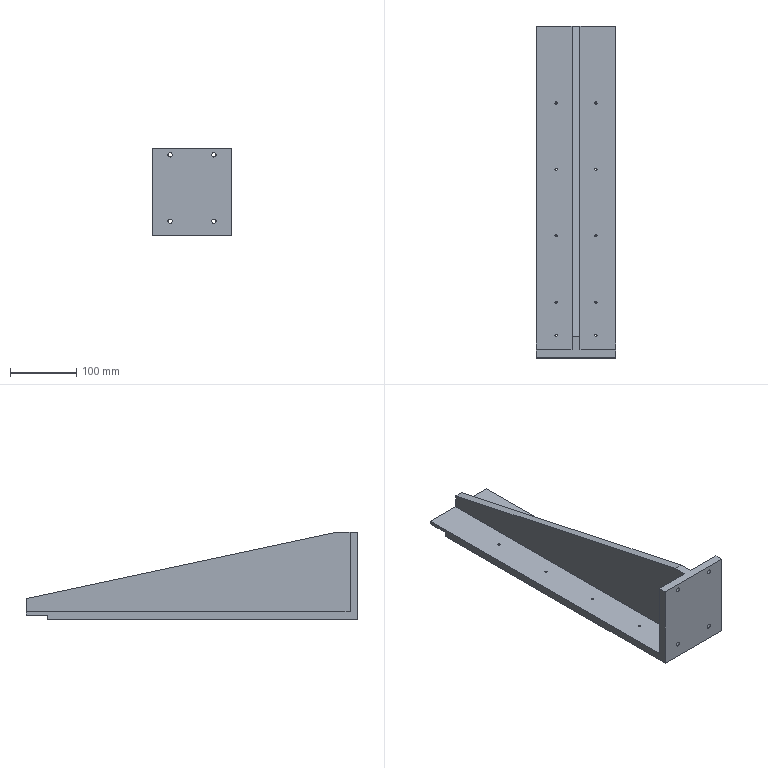Part | SolidWorks | features HoleWzd 3, ICE 2, Cut 1, Extrusion 1 | 1 solid | 43 faces | box 120 x 500 x 132 mm | volume 1285339 mm3 | cylinder 28 | plane 15 | commonest cylinder face diameters 3.3 x20 6.6 x8
STEP:
#1=CARTESIAN_POINT('',(28.35,34.,12.));
#2=VERTEX_POINT('',#1);
#3=CARTESIAN_POINT('',(31.65,34.,12.));
#4=VERTEX_POINT('',#3);
#5=CARTESIAN_POINT('',(30.,34.,12.));
#6=DIRECTION('',(0.,0.,1.));
#7=DIRECTION('',(1.,0.,0.));
#8=AXIS2_PLACEMENT_3D('',#5,#6,#7);
#9=CIRCLE('',#8,1.65);
#10=EDGE_CURVE('',#2,#4,#9,.T.);
#11=ORIENTED_EDGE('',*,*,#10,.T.);
#12=CARTESIAN_POINT('',(31.65,34.,0.));
#13=VERTEX_POINT('',#12);
#14=CARTESIAN_POINT('',(31.65,34.,0.));
#15=DIRECTION('',(0.,0.,-1.));
#16=VECTOR('',#15,1000.);
#17=LINE('',#14,#16);
#18=EDGE_CURVE('',#4,#13,#17,.T.);
#19=ORIENTED_EDGE('',*,*,#18,.T.);
#20=CARTESIAN_POINT('',(28.35,34.,0.));
#21=VERTEX_POINT('',#20);
#22=CARTESIAN_POINT('',(30.,34.,0.));
#23=DIRECTION('',(0.,0.,-1.));
#24=DIRECTION('',(-1.,0.,0.));
#25=AXIS2_PLACEMENT_3D('',#22,#23,#24);
#26=CIRCLE('',#25,1.65);
#27=EDGE_CURVE('',#13,#21,#26,.T.);
#28=ORIENTED_EDGE('',*,*,#27,.T.);
#29=CARTESIAN_POINT('',(28.35,34.,0.));
#30=DIRECTION('',(0.,0.,-1.));
#31=VECTOR('',#30,1000.);
#32=LINE('',#29,#31);
#33=EDGE_CURVE('',#2,#21,#32,.T.);
#34=ORIENTED_EDGE('',*,*,#33,.F.);
#35=EDGE_LOOP('',(#11,#19,#28,#34));
#36=FACE_OUTER_BOUND('',#35,.T.);
#37=CARTESIAN_POINT('',(30.,34.,0.));
#38=DIRECTION('',(0.,0.,-1.));
#39=DIRECTION('',(-1.,0.,0.));
#40=AXIS2_PLACEMENT_3D('',#37,#38,#39);
#41=CYLINDRICAL_SURFACE('',#40,1.65);
#42=ADVANCED_FACE('',(#36),#41,.F.);
#43=CARTESIAN_POINT('',(28.35,134.,12.));
#44=VERTEX_POINT('',#43);
#45=CARTESIAN_POINT('',(31.65,134.,12.));
#46=VERTEX_POINT('',#45);
#47=CARTESIAN_POINT('',(30.,134.,12.));
#48=DIRECTION('',(0.,0.,1.));
#49=DIRECTION('',(1.,0.,0.));
#50=AXIS2_PLACEMENT_3D('',#47,#48,#49);
#51=CIRCLE('',#50,1.65);
#52=EDGE_CURVE('',#44,#46,#51,.T.);
#53=ORIENTED_EDGE('',*,*,#52,.T.);
#54=CARTESIAN_POINT('',(31.65,134.,0.));
#55=VERTEX_POINT('',#54);
#56=CARTESIAN_POINT('',(31.65,134.,0.));
#57=DIRECTION('',(0.,0.,-1.));
#58=VECTOR('',#57,1000.);
#59=LINE('',#56,#58);
#60=EDGE_CURVE('',#46,#55,#59,.T.);
#61=ORIENTED_EDGE('',*,*,#60,.T.);
#62=CARTESIAN_POINT('',(28.35,134.,0.));
#63=VERTEX_POINT('',#62);
#64=CARTESIAN_POINT('',(30.,134.,0.));
#65=DIRECTION('',(0.,0.,-1.));
#66=DIRECTION('',(-1.,0.,0.));
#67=AXIS2_PLACEMENT_3D('',#64,#65,#66);
#68=CIRCLE('',#67,1.65);
#69=EDGE_CURVE('',#55,#63,#68,.T.);
#70=ORIENTED_EDGE('',*,*,#69,.T.);
#71=CARTESIAN_POINT('',(28.35,134.,0.));
#72=DIRECTION('',(0.,0.,-1.));
#73=VECTOR('',#72,1000.);
#74=LINE('',#71,#73);
#75=EDGE_CURVE('',#44,#63,#74,.T.);
#76=ORIENTED_EDGE('',*,*,#75,.F.);
#77=EDGE_LOOP('',(#53,#61,#70,#76));
#78=FACE_OUTER_BOUND('',#77,.T.);
#79=CARTESIAN_POINT('',(30.,134.,0.));
#80=DIRECTION('',(0.,0.,-1.));
#81=DIRECTION('',(-1.,0.,0.));
#82=AXIS2_PLACEMENT_3D('',#79,#80,#81);
#83=CYLINDRICAL_SURFACE('',#82,1.65);
#84=ADVANCED_FACE('',(#78),#83,.F.);
#85=CARTESIAN_POINT('',(28.35,-66.,12.));
#86=VERTEX_POINT('',#85);
#87=CARTESIAN_POINT('',(31.65,-66.,12.));
#88=VERTEX_POINT('',#87);
#89=CARTESIAN_POINT('',(30.,-66.,12.));
#90=DIRECTION('',(0.,0.,1.));
#91=DIRECTION('',(1.,0.,0.));
#92=AXIS2_PLACEMENT_3D('',#89,#90,#91);
#93=CIRCLE('',#92,1.65);
#94=EDGE_CURVE('',#86,#88,#93,.T.);
#95=ORIENTED_EDGE('',*,*,#94,.T.);
#96=CARTESIAN_POINT('',(31.65,-66.,0.));
#97=VERTEX_POINT('',#96);
#98=CARTESIAN_POINT('',(31.65,-66.,0.));
#99=DIRECTION('',(0.,0.,-1.));
#100=VECTOR('',#99,1000.);
#101=LINE('',#98,#100);
#102=EDGE_CURVE('',#88,#97,#101,.T.);
#103=ORIENTED_EDGE('',*,*,#102,.T.);
#104=CARTESIAN_POINT('',(28.35,-66.,0.));
#105=VERTEX_POINT('',#104);
#106=CARTESIAN_POINT('',(30.,-66.,0.));
#107=DIRECTION('',(0.,0.,-1.));
#108=DIRECTION('',(-1.,0.,0.));
#109=AXIS2_PLACEMENT_3D('',#106,#107,#108);
#110=CIRCLE('',#109,1.65);
#111=EDGE_CURVE('',#97,#105,#110,.T.);
#112=ORIENTED_EDGE('',*,*,#111,.T.);
#113=CARTESIAN_POINT('',(28.35,-66.,0.));
#114=DIRECTION('',(0.,0.,-1.));
#115=VECTOR('',#114,1000.);
#116=LINE('',#113,#115);
#117=EDGE_CURVE('',#86,#105,#116,.T.);
#118=ORIENTED_EDGE('',*,*,#117,.F.);
#119=EDGE_LOOP('',(#95,#103,#112,#118));
#120=FACE_OUTER_BOUND('',#119,.T.);
#121=CARTESIAN_POINT('',(30.,-66.,0.));
#122=DIRECTION('',(0.,0.,-1.));
#123=DIRECTION('',(-1.,0.,0.));
#124=AXIS2_PLACEMENT_3D('',#121,#122,#123);
#125=CYLINDRICAL_SURFACE('',#124,1.65);
#126=ADVANCED_FACE('',(#120),#125,.F.);
#127=CARTESIAN_POINT('',(28.35,-166.,12.));
#128=VERTEX_POINT('',#127);
#129=CARTESIAN_POINT('',(31.65,-166.,12.));
#130=VERTEX_POINT('',#129);
#131=CARTESIAN_POINT('',(30.,-166.,12.));
#132=DIRECTION('',(0.,0.,1.));
#133=DIRECTION('',(1.,0.,0.));
#134=AXIS2_PLACEMENT_3D('',#131,#132,#133);
#135=CIRCLE('',#134,1.65);
#136=EDGE_CURVE('',#128,#130,#135,.T.);
#137=ORIENTED_EDGE('',*,*,#136,.T.);
#138=CARTESIAN_POINT('',(31.65,-166.,0.));
#139=VERTEX_POINT('',#138);
#140=CARTESIAN_POINT('',(31.65,-166.,0.));
#141=DIRECTION('',(0.,0.,-1.));
#142=VECTOR('',#141,1000.);
#143=LINE('',#140,#142);
#144=EDGE_CURVE('',#130,#139,#143,.T.);
#145=ORIENTED_EDGE('',*,*,#144,.T.);
#146=CARTESIAN_POINT('',(28.35,-166.,0.));
#147=VERTEX_POINT('',#146);
#148=CARTESIAN_POINT('',(30.,-166.,0.));
#149=DIRECTION('',(0.,0.,-1.));
#150=DIRECTION('',(-1.,0.,0.));
#151=AXIS2_PLACEMENT_3D('',#148,#149,#150);
#152=CIRCLE('',#151,1.65);
#153=EDGE_CURVE('',#139,#147,#152,.T.);
#154=ORIENTED_EDGE('',*,*,#153,.T.);
#155=CARTESIAN_POINT('',(28.35,-166.,0.));
#156=DIRECTION('',(0.,0.,-1.));
#157=VECTOR('',#156,1000.);
#158=LINE('',#155,#157);
#159=EDGE_CURVE('',#128,#147,#158,.T.);
#160=ORIENTED_EDGE('',*,*,#159,.F.);
#161=EDGE_LOOP('',(#137,#145,#154,#160));
#162=FACE_OUTER_BOUND('',#161,.T.);
#163=CARTESIAN_POINT('',(30.,-166.,0.));
#164=DIRECTION('',(0.,0.,-1.));
#165=DIRECTION('',(-1.,0.,0.));
#166=AXIS2_PLACEMENT_3D('',#163,#164,#165);
#167=CYLINDRICAL_SURFACE('',#166,1.65);
#168=ADVANCED_FACE('',(#162),#167,.F.);
#169=CARTESIAN_POINT('',(28.35,-216.,12.));
#170=VERTEX_POINT('',#169);
#171=CARTESIAN_POINT('',(31.65,-216.,12.));
#172=VERTEX_POINT('',#171);
#173=CARTESIAN_POINT('',(30.,-216.,12.));
#174=DIRECTION('',(0.,0.,1.));
#175=DIRECTION('',(1.,0.,0.));
#176=AXIS2_PLACEMENT_3D('',#173,#174,#175);
#177=CIRCLE('',#176,1.65);
#178=EDGE_CURVE('',#170,#172,#177,.T.);
#179=ORIENTED_EDGE('',*,*,#178,.T.);
#180=CARTESIAN_POINT('',(31.65,-216.,0.));
#181=VERTEX_POINT('',#180);
#182=CARTESIAN_POINT('',(31.65,-216.,0.));
#183=DIRECTION('',(0.,0.,-1.));
#184=VECTOR('',#183,1000.);
#185=LINE('',#182,#184);
#186=EDGE_CURVE('',#172,#181,#185,.T.);
#187=ORIENTED_EDGE('',*,*,#186,.T.);
#188=CARTESIAN_POINT('',(28.35,-216.,0.));
#189=VERTEX_POINT('',#188);
#190=CARTESIAN_POINT('',(30.,-216.,0.));
#191=DIRECTION('',(0.,0.,-1.));
#192=DIRECTION('',(-1.,0.,0.));
#193=AXIS2_PLACEMENT_3D('',#190,#191,#192);
#194=CIRCLE('',#193,1.65);
#195=EDGE_CURVE('',#181,#189,#194,.T.);
#196=ORIENTED_EDGE('',*,*,#195,.T.);
#197=CARTESIAN_POINT('',(28.35,-216.,0.));
#198=DIRECTION('',(0.,0.,-1.));
#199=VECTOR('',#198,1000.);
#200=LINE('',#197,#199);
#201=EDGE_CURVE('',#170,#189,#200,.T.);
#202=ORIENTED_EDGE('',*,*,#201,.F.);
#203=EDGE_LOOP('',(#179,#187,#196,#202));
#204=FACE_OUTER_BOUND('',#203,.T.);
#205=CARTESIAN_POINT('',(30.,-216.,0.));
#206=DIRECTION('',(0.,0.,-1.));
#207=DIRECTION('',(-1.,0.,0.));
#208=AXIS2_PLACEMENT_3D('',#205,#206,#207);
#209=CYLINDRICAL_SURFACE('',#208,1.65);
#210=ADVANCED_FACE('',(#204),#209,.F.);
#211=CARTESIAN_POINT('',(-31.65,-216.,12.));
#212=VERTEX_POINT('',#211);
#213=CARTESIAN_POINT('',(-28.35,-216.,12.));
#214=VERTEX_POINT('',#213);
#215=CARTESIAN_POINT('',(-30.,-216.,12.));
#216=DIRECTION('',(0.,0.,1.));
#217=DIRECTION('',(1.,0.,0.));
#218=AXIS2_PLACEMENT_3D('',#215,#216,#217);
#219=CIRCLE('',#218,1.65);
#220=EDGE_CURVE('',#212,#214,#219,.T.);
#221=ORIENTED_EDGE('',*,*,#220,.T.);
#222=CARTESIAN_POINT('',(-28.35,-216.,0.));
#223=VERTEX_POINT('',#222);
#224=CARTESIAN_POINT('',(-28.35,-216.,0.));
#225=DIRECTION('',(0.,0.,-1.));
#226=VECTOR('',#225,1000.);
#227=LINE('',#224,#226);
#228=EDGE_CURVE('',#214,#223,#227,.T.);
#229=ORIENTED_EDGE('',*,*,#228,.T.);
#230=CARTESIAN_POINT('',(-31.65,-216.,0.));
#231=VERTEX_POINT('',#230);
#232=CARTESIAN_POINT('',(-30.,-216.,0.));
#233=DIRECTION('',(0.,0.,-1.));
#234=DIRECTION('',(-1.,0.,0.));
#235=AXIS2_PLACEMENT_3D('',#232,#233,#234);
#236=CIRCLE('',#235,1.65);
#237=EDGE_CURVE('',#223,#231,#236,.T.);
#238=ORIENTED_EDGE('',*,*,#237,.T.);
#239=CARTESIAN_POINT('',(-31.65,-216.,0.));
#240=DIRECTION('',(0.,0.,-1.));
#241=VECTOR('',#240,1000.);
#242=LINE('',#239,#241);
#243=EDGE_CURVE('',#212,#231,#242,.T.);
#244=ORIENTED_EDGE('',*,*,#243,.F.);
#245=EDGE_LOOP('',(#221,#229,#238,#244));
#246=FACE_OUTER_BOUND('',#245,.T.);
#247=CARTESIAN_POINT('',(-30.,-216.,0.));
#248=DIRECTION('',(0.,0.,-1.));
#249=DIRECTION('',(-1.,0.,0.));
#250=AXIS2_PLACEMENT_3D('',#247,#248,#249);
#251=CYLINDRICAL_SURFACE('',#250,1.65);
#252=ADVANCED_FACE('',(#246),#251,.F.);
#253=CARTESIAN_POINT('',(-31.65,-166.,12.));
#254=VERTEX_POINT('',#253);
#255=CARTESIAN_POINT('',(-28.35,-166.,12.));
#256=VERTEX_POINT('',#255);
#257=CARTESIAN_POINT('',(-30.,-166.,12.));
#258=DIRECTION('',(0.,0.,1.));
#259=DIRECTION('',(1.,0.,0.));
#260=AXIS2_PLACEMENT_3D('',#257,#258,#259);
#261=CIRCLE('',#260,1.65);
#262=EDGE_CURVE('',#254,#256,#261,.T.);
#263=ORIENTED_EDGE('',*,*,#262,.T.);
#264=CARTESIAN_POINT('',(-28.35,-166.,0.));
#265=VERTEX_POINT('',#264);
#266=CARTESIAN_POINT('',(-28.35,-166.,0.));
#267=DIRECTION('',(0.,0.,-1.));
#268=VECTOR('',#267,1000.);
#269=LINE('',#266,#268);
#270=EDGE_CURVE('',#256,#265,#269,.T.);
#271=ORIENTED_EDGE('',*,*,#270,.T.);
#272=CARTESIAN_POINT('',(-31.65,-166.,0.));
#273=VERTEX_POINT('',#272);
#274=CARTESIAN_POINT('',(-30.,-166.,0.));
#275=DIRECTION('',(0.,0.,-1.));
#276=DIRECTION('',(-1.,0.,0.));
#277=AXIS2_PLACEMENT_3D('',#274,#275,#276);
#278=CIRCLE('',#277,1.65);
#279=EDGE_CURVE('',#265,#273,#278,.T.);
#280=ORIENTED_EDGE('',*,*,#279,.T.);
#281=CARTESIAN_POINT('',(-31.65,-166.,0.));
#282=DIRECTION('',(0.,0.,-1.));
#283=VECTOR('',#282,1000.);
#284=LINE('',#281,#283);
#285=EDGE_CURVE('',#254,#273,#284,.T.);
#286=ORIENTED_EDGE('',*,*,#285,.F.);
#287=EDGE_LOOP('',(#263,#271,#280,#286));
#288=FACE_OUTER_BOUND('',#287,.T.);
#289=CARTESIAN_POINT('',(-30.,-166.,0.));
#290=DIRECTION('',(0.,0.,-1.));
#291=DIRECTION('',(-1.,0.,0.));
#292=AXIS2_PLACEMENT_3D('',#289,#290,#291);
#293=CYLINDRICAL_SURFACE('',#292,1.65);
#294=ADVANCED_FACE('',(#288),#293,.F.);
#295=CARTESIAN_POINT('',(-31.65,-66.,12.));
#296=VERTEX_POINT('',#295);
#297=CARTESIAN_POINT('',(-28.35,-66.,12.));
#298=VERTEX_POINT('',#297);
#299=CARTESIAN_POINT('',(-30.,-66.,12.));
#300=DIRECTION('',(0.,0.,1.));
#301=DIRECTION('',(1.,0.,0.));
#302=AXIS2_PLACEMENT_3D('',#299,#300,#301);
#303=CIRCLE('',#302,1.65);
#304=EDGE_CURVE('',#296,#298,#303,.T.);
#305=ORIENTED_EDGE('',*,*,#304,.T.);
#306=CARTESIAN_POINT('',(-28.35,-66.,0.));
#307=VERTEX_POINT('',#306);
#308=CARTESIAN_POINT('',(-28.35,-66.,0.));
#309=DIRECTION('',(0.,0.,-1.));
#310=VECTOR('',#309,1000.);
#311=LINE('',#308,#310);
#312=EDGE_CURVE('',#298,#307,#311,.T.);
#313=ORIENTED_EDGE('',*,*,#312,.T.);
#314=CARTESIAN_POINT('',(-31.65,-66.,0.));
#315=VERTEX_POINT('',#314);
#316=CARTESIAN_POINT('',(-30.,-66.,0.));
#317=DIRECTION('',(0.,0.,-1.));
#318=DIRECTION('',(-1.,0.,0.));
#319=AXIS2_PLACEMENT_3D('',#316,#317,#318);
#320=CIRCLE('',#319,1.65);
#321=EDGE_CURVE('',#307,#315,#320,.T.);
#322=ORIENTED_EDGE('',*,*,#321,.T.);
#323=CARTESIAN_POINT('',(-31.65,-66.,0.));
#324=DIRECTION('',(0.,0.,-1.));
#325=VECTOR('',#324,1000.);
#326=LINE('',#323,#325);
#327=EDGE_CURVE('',#296,#315,#326,.T.);
#328=ORIENTED_EDGE('',*,*,#327,.F.);
#329=EDGE_LOOP('',(#305,#313,#322,#328));
#330=FACE_OUTER_BOUND('',#329,.T.);
#331=CARTESIAN_POINT('',(-30.,-66.,0.));
#332=DIRECTION('',(0.,0.,-1.));
#333=DIRECTION('',(-1.,0.,0.));
#334=AXIS2_PLACEMENT_3D('',#331,#332,#333);
#335=CYLINDRICAL_SURFACE('',#334,1.65);
#336=ADVANCED_FACE('',(#330),#335,.F.);
#337=CARTESIAN_POINT('',(-31.65,34.,12.));
#338=VERTEX_POINT('',#337);
#339=CARTESIAN_POINT('',(-28.35,34.,12.));
#340=VERTEX_POINT('',#339);
#341=CARTESIAN_POINT('',(-30.,34.,12.));
#342=DIRECTION('',(0.,0.,1.));
#343=DIRECTION('',(1.,0.,0.));
#344=AXIS2_PLACEMENT_3D('',#341,#342,#343);
#345=CIRCLE('',#344,1.65);
#346=EDGE_CURVE('',#338,#340,#345,.T.);
#347=ORIENTED_EDGE('',*,*,#346,.T.);
#348=CARTESIAN_POINT('',(-28.35,34.,0.));
#349=VERTEX_POINT('',#348);
#350=CARTESIAN_POINT('',(-28.35,34.,0.));
#351=DIRECTION('',(0.,0.,-1.));
#352=VECTOR('',#351,1000.);
#353=LINE('',#350,#352);
#354=EDGE_CURVE('',#340,#349,#353,.T.);
#355=ORIENTED_EDGE('',*,*,#354,.T.);
#356=CARTESIAN_POINT('',(-31.65,34.,0.));
#357=VERTEX_POINT('',#356);
#358=CARTESIAN_POINT('',(-30.,34.,0.));
#359=DIRECTION('',(0.,0.,-1.));
#360=DIRECTION('',(-1.,0.,0.));
#361=AXIS2_PLACEMENT_3D('',#358,#359,#360);
#362=CIRCLE('',#361,1.65);
#363=EDGE_CURVE('',#349,#357,#362,.T.);
#364=ORIENTED_EDGE('',*,*,#363,.T.);
#365=CARTESIAN_POINT('',(-31.65,34.,0.));
#366=DIRECTION('',(0.,0.,-1.));
#367=VECTOR('',#366,1000.);
#368=LINE('',#365,#367);
#369=EDGE_CURVE('',#338,#357,#368,.T.);
#370=ORIENTED_EDGE('',*,*,#369,.F.);
#371=EDGE_LOOP('',(#347,#355,#364,#370));
#372=FACE_OUTER_BOUND('',#371,.T.);
#373=CARTESIAN_POINT('',(-30.,34.,0.));
#374=DIRECTION('',(0.,0.,-1.));
#375=DIRECTION('',(-1.,0.,0.));
#376=AXIS2_PLACEMENT_3D('',#373,#374,#375);
#377=CYLINDRICAL_SURFACE('',#376,1.65);
#378=ADVANCED_FACE('',(#372),#377,.F.);
#379=CARTESIAN_POINT('',(-31.65,134.,12.));
#380=VERTEX_POINT('',#379);
#381=CARTESIAN_POINT('',(-28.35,134.,12.));
#382=VERTEX_POINT('',#381);
#383=CARTESIAN_POINT('',(-30.,134.,12.));
#384=DIRECTION('',(0.,0.,1.));
#385=DIRECTION('',(1.,0.,0.));
#386=AXIS2_PLACEMENT_3D('',#383,#384,#385);
#387=CIRCLE('',#386,1.65);
#388=EDGE_CURVE('',#380,#382,#387,.T.);
#389=ORIENTED_EDGE('',*,*,#388,.T.);
#390=CARTESIAN_POINT('',(-28.35,134.,0.));
#391=VERTEX_POINT('',#390);
#392=CARTESIAN_POINT('',(-28.35,134.,0.));
#393=DIRECTION('',(0.,0.,-1.));
#394=VECTOR('',#393,1000.);
#395=LINE('',#392,#394);
#396=EDGE_CURVE('',#382,#391,#395,.T.);
#397=ORIENTED_EDGE('',*,*,#396,.T.);
#398=CARTESIAN_POINT('',(-31.65,134.,0.));
#399=VERTEX_POINT('',#398);
#400=CARTESIAN_POINT('',(-30.,134.,0.));
#401=DIRECTION('',(0.,0.,-1.));
#402=DIRECTION('',(-1.,0.,0.));
#403=AXIS2_PLACEMENT_3D('',#400,#401,#402);
#404=CIRCLE('',#403,1.65);
#405=EDGE_CURVE('',#391,#399,#404,.T.);
#406=ORIENTED_EDGE('',*,*,#405,.T.);
#407=CARTESIAN_POINT('',(-31.65,134.,0.));
#408=DIRECTION('',(0.,0.,-1.));
#409=VECTOR('',#408,1000.);
#410=LINE('',#407,#409);
#411=EDGE_CURVE('',#380,#399,#410,.T.);
#412=ORIENTED_EDGE('',*,*,#411,.F.);
#413=EDGE_LOOP('',(#389,#397,#406,#412));
#414=FACE_OUTER_BOUND('',#413,.T.);
#415=CARTESIAN_POINT('',(-30.,134.,0.));
#416=DIRECTION('',(0.,0.,-1.));
#417=DIRECTION('',(-1.,0.,0.));
#418=AXIS2_PLACEMENT_3D('',#415,#416,#417);
#419=CYLINDRICAL_SURFACE('',#418,1.65);
#420=ADVANCED_FACE('',(#414),#419,.F.);
#421=CARTESIAN_POINT('',(-33.,-250.,18.7));
#422=VERTEX_POINT('',#421);
#423=CARTESIAN_POINT('',(-33.,-250.,25.3));
#424=VERTEX_POINT('',#423);
#425=CARTESIAN_POINT('',(-33.,-250.,22.));
#426=DIRECTION('',(0.,1.,0.));
#427=DIRECTION('',(0.,0.,1.));
#428=AXIS2_PLACEMENT_3D('',#425,#426,#427);
#429=CIRCLE('',#428,3.3);
#430=EDGE_CURVE('',#422,#424,#429,.T.);
#431=ORIENTED_EDGE('',*,*,#430,.F.);
#432=CARTESIAN_POINT('',(-33.,-238.,18.7));
#433=VERTEX_POINT('',#432);
#434=CARTESIAN_POINT('',(-33.,-238.,18.7));
#435=DIRECTION('',(0.,1.,0.));
#436=VECTOR('',#435,1000.);
#437=LINE('',#434,#436);
#438=EDGE_CURVE('',#422,#433,#437,.T.);
#439=ORIENTED_EDGE('',*,*,#438,.T.);
#440=CARTESIAN_POINT('',(-33.,-238.,25.3));
#441=VERTEX_POINT('',#440);
#442=CARTESIAN_POINT('',(-33.,-238.,22.));
#443=DIRECTION('',(0.,1.,0.));
#444=DIRECTION('',(0.,0.,1.));
#445=AXIS2_PLACEMENT_3D('',#442,#443,#444);
#446=CIRCLE('',#445,3.3);
#447=EDGE_CURVE('',#433,#441,#446,.T.);
#448=ORIENTED_EDGE('',*,*,#447,.T.);
#449=CARTESIAN_POINT('',(-33.,-238.,25.3));
#450=DIRECTION('',(0.,1.,0.));
#451=VECTOR('',#450,1000.);
#452=LINE('',#449,#451);
#453=EDGE_CURVE('',#424,#441,#452,.T.);
#454=ORIENTED_EDGE('',*,*,#453,.F.);
#455=EDGE_LOOP('',(#431,#439,#448,#454));
#456=FACE_OUTER_BOUND('',#455,.T.);
#457=CARTESIAN_POINT('',(-33.,-238.,22.));
#458=DIRECTION('',(0.,1.,0.));
#459=DIRECTION('',(0.,0.,1.));
#460=AXIS2_PLACEMENT_3D('',#457,#458,#459);
#461=CYLINDRICAL_SURFACE('',#460,3.3);
#462=ADVANCED_FACE('',(#456),#461,.F.);
#463=CARTESIAN_POINT('',(-33.,-250.,118.7));
#464=VERTEX_POINT('',#463);
#465=CARTESIAN_POINT('',(-33.,-250.,125.3));
#466=VERTEX_POINT('',#465);
#467=CARTESIAN_POINT('',(-33.,-250.,122.));
#468=DIRECTION('',(0.,1.,0.));
#469=DIRECTION('',(0.,0.,1.));
#470=AXIS2_PLACEMENT_3D('',#467,#468,#469);
#471=CIRCLE('',#470,3.3);
#472=EDGE_CURVE('',#464,#466,#471,.T.);
#473=ORIENTED_EDGE('',*,*,#472,.F.);
#474=CARTESIAN_POINT('',(-33.,-238.,118.7));
#475=VERTEX_POINT('',#474);
#476=CARTESIAN_POINT('',(-33.,-238.,118.7));
#477=DIRECTION('',(0.,1.,0.));
#478=VECTOR('',#477,1000.);
#479=LINE('',#476,#478);
#480=EDGE_CURVE('',#464,#475,#479,.T.);
#481=ORIENTED_EDGE('',*,*,#480,.T.);
#482=CARTESIAN_POINT('',(-33.,-238.,125.3));
#483=VERTEX_POINT('',#482);
#484=CARTESIAN_POINT('',(-33.,-238.,122.));
#485=DIRECTION('',(0.,1.,0.));
#486=DIRECTION('',(0.,0.,1.));
#487=AXIS2_PLACEMENT_3D('',#484,#485,#486);
#488=CIRCLE('',#487,3.3);
#489=EDGE_CURVE('',#475,#483,#488,.T.);
#490=ORIENTED_EDGE('',*,*,#489,.T.);
#491=CARTESIAN_POINT('',(-33.,-238.,125.3));
#492=DIRECTION('',(0.,1.,0.));
#493=VECTOR('',#492,1000.);
#494=LINE('',#491,#493);
#495=EDGE_CURVE('',#466,#483,#494,.T.);
#496=ORIENTED_EDGE('',*,*,#495,.F.);
#497=EDGE_LOOP('',(#473,#481,#490,#496));
#498=FACE_OUTER_BOUND('',#497,.T.);
#499=CARTESIAN_POINT('',(-33.,-238.,122.));
#500=DIRECTION('',(0.,1.,0.));
#501=DIRECTION('',(0.,0.,1.));
#502=AXIS2_PLACEMENT_3D('',#499,#500,#501);
#503=CYLINDRICAL_SURFACE('',#502,3.3);
#504=ADVANCED_FACE('',(#498),#503,.F.);
#505=CARTESIAN_POINT('',(33.,-250.,18.7));
#506=VERTEX_POINT('',#505);
#507=CARTESIAN_POINT('',(33.,-250.,25.3));
#508=VERTEX_POINT('',#507);
#509=CARTESIAN_POINT('',(33.,-250.,22.));
#510=DIRECTION('',(0.,1.,0.));
#511=DIRECTION('',(0.,0.,1.));
#512=AXIS2_PLACEMENT_3D('',#509,#510,#511);
#513=CIRCLE('',#512,3.3);
#514=EDGE_CURVE('',#506,#508,#513,.T.);
#515=ORIENTED_EDGE('',*,*,#514,.F.);
#516=CARTESIAN_POINT('',(33.,-238.,18.7));
#517=VERTEX_POINT('',#516);
#518=CARTESIAN_POINT('',(33.,-238.,18.7));
#519=DIRECTION('',(0.,1.,0.));
#520=VECTOR('',#519,1000.);
#521=LINE('',#518,#520);
#522=EDGE_CURVE('',#506,#517,#521,.T.);
#523=ORIENTED_EDGE('',*,*,#522,.T.);
#524=CARTESIAN_POINT('',(33.,-238.,25.3));
#525=VERTEX_POINT('',#524);
#526=CARTESIAN_POINT('',(33.,-238.,22.));
#527=DIRECTION('',(0.,1.,0.));
#528=DIRECTION('',(0.,0.,1.));
#529=AXIS2_PLACEMENT_3D('',#526,#527,#528);
#530=CIRCLE('',#529,3.3);
#531=EDGE_CURVE('',#517,#525,#530,.T.);
#532=ORIENTED_EDGE('',*,*,#531,.T.);
#533=CARTESIAN_POINT('',(33.,-238.,25.3));
#534=DIRECTION('',(0.,1.,0.));
#535=VECTOR('',#534,1000.);
#536=LINE('',#533,#535);
#537=EDGE_CURVE('',#508,#525,#536,.T.);
#538=ORIENTED_EDGE('',*,*,#537,.F.);
#539=EDGE_LOOP('',(#515,#523,#532,#538));
#540=FACE_OUTER_BOUND('',#539,.T.);
#541=CARTESIAN_POINT('',(33.,-238.,22.));
#542=DIRECTION('',(0.,1.,0.));
#543=DIRECTION('',(0.,0.,1.));
#544=AXIS2_PLACEMENT_3D('',#541,#542,#543);
#545=CYLINDRICAL_SURFACE('',#544,3.3);
#546=ADVANCED_FACE('',(#540),#545,.F.);
#547=CARTESIAN_POINT('',(33.,-250.,118.7));
#548=VERTEX_POINT('',#547);
#549=CARTESIAN_POINT('',(33.,-250.,125.3));
#550=VERTEX_POINT('',#549);
#551=CARTESIAN_POINT('',(33.,-250.,122.));
#552=DIRECTION('',(0.,1.,0.));
#553=DIRECTION('',(0.,0.,1.));
#554=AXIS2_PLACEMENT_3D('',#551,#552,#553);
#555=CIRCLE('',#554,3.3);
#556=EDGE_CURVE('',#548,#550,#555,.T.);
#557=ORIENTED_EDGE('',*,*,#556,.F.);
#558=CARTESIAN_POINT('',(33.,-238.,118.7));
#559=VERTEX_POINT('',#558);
#560=CARTESIAN_POINT('',(33.,-238.,118.7));
#561=DIRECTION('',(0.,1.,0.));
#562=VECTOR('',#561,1000.);
#563=LINE('',#560,#562);
#564=EDGE_CURVE('',#548,#559,#563,.T.);
#565=ORIENTED_EDGE('',*,*,#564,.T.);
#566=CARTESIAN_POINT('',(33.,-238.,125.3));
#567=VERTEX_POINT('',#566);
#568=CARTESIAN_POINT('',(33.,-238.,122.));
#569=DIRECTION('',(0.,1.,0.));
#570=DIRECTION('',(0.,0.,1.));
#571=AXIS2_PLACEMENT_3D('',#568,#569,#570);
#572=CIRCLE('',#571,3.3);
#573=EDGE_CURVE('',#559,#567,#572,.T.);
#574=ORIENTED_EDGE('',*,*,#573,.T.);
#575=CARTESIAN_POINT('',(33.,-238.,125.3));
#576=DIRECTION('',(0.,1.,0.));
#577=VECTOR('',#576,1000.);
#578=LINE('',#575,#577);
#579=EDGE_CURVE('',#550,#567,#578,.T.);
#580=ORIENTED_EDGE('',*,*,#579,.F.);
#581=EDGE_LOOP('',(#557,#565,#574,#580));
#582=FACE_OUTER_BOUND('',#581,.T.);
#583=CARTESIAN_POINT('',(33.,-238.,122.));
#584=DIRECTION('',(0.,1.,0.));
#585=DIRECTION('',(0.,0.,1.));
#586=AXIS2_PLACEMENT_3D('',#583,#584,#585);
#587=CYLINDRICAL_SURFACE('',#586,3.3);
#588=ADVANCED_FACE('',(#582),#587,.F.);
#589=ORIENTED_EDGE('',*,*,#220,.F.);
#590=CARTESIAN_POINT('',(-30.,-216.,12.));
#591=DIRECTION('',(0.,0.,1.));
#592=DIRECTION('',(1.,0.,0.));
#593=AXIS2_PLACEMENT_3D('',#590,#591,#592);
#594=CIRCLE('',#593,1.65);
#595=EDGE_CURVE('',#214,#212,#594,.T.);
#596=ORIENTED_EDGE('',*,*,#595,.F.);
#597=EDGE_LOOP('',(#589,#596));
#598=FACE_BOUND('',#597,.T.);
#599=ORIENTED_EDGE('',*,*,#262,.F.);
#600=CARTESIAN_POINT('',(-30.,-166.,12.));
#601=DIRECTION('',(0.,0.,1.));
#602=DIRECTION('',(1.,0.,0.));
#603=AXIS2_PLACEMENT_3D('',#600,#601,#602);
#604=CIRCLE('',#603,1.65);
#605=EDGE_CURVE('',#256,#254,#604,.T.);
#606=ORIENTED_EDGE('',*,*,#605,.F.);
#607=EDGE_LOOP('',(#599,#606));
#608=FACE_BOUND('',#607,.T.);
#609=ORIENTED_EDGE('',*,*,#304,.F.);
#610=CARTESIAN_POINT('',(-30.,-66.,12.));
#611=DIRECTION('',(0.,0.,1.));
#612=DIRECTION('',(1.,0.,0.));
#613=AXIS2_PLACEMENT_3D('',#610,#611,#612);
#614=CIRCLE('',#613,1.65);
#615=EDGE_CURVE('',#298,#296,#614,.T.);
#616=ORIENTED_EDGE('',*,*,#615,.F.);
#617=EDGE_LOOP('',(#609,#616));
#618=FACE_BOUND('',#617,.T.);
#619=ORIENTED_EDGE('',*,*,#346,.F.);
#620=CARTESIAN_POINT('',(-30.,34.,12.));
#621=DIRECTION('',(0.,0.,1.));
#622=DIRECTION('',(1.,0.,0.));
#623=AXIS2_PLACEMENT_3D('',#620,#621,#622);
#624=CIRCLE('',#623,1.65);
#625=EDGE_CURVE('',#340,#338,#624,.T.);
#626=ORIENTED_EDGE('',*,*,#625,.F.);
#627=EDGE_LOOP('',(#619,#626));
#628=FACE_BOUND('',#627,.T.);
#629=ORIENTED_EDGE('',*,*,#388,.F.);
#630=CARTESIAN_POINT('',(-30.,134.,12.));
#631=DIRECTION('',(0.,0.,1.));
#632=DIRECTION('',(1.,0.,0.));
#633=AXIS2_PLACEMENT_3D('',#630,#631,#632);
#634=CIRCLE('',#633,1.65);
#635=EDGE_CURVE('',#382,#380,#634,.T.);
#636=ORIENTED_EDGE('',*,*,#635,.F.);
#637=EDGE_LOOP('',(#629,#636));
#638=FACE_BOUND('',#637,.T.);
#639=CARTESIAN_POINT('',(-6.,-238.,12.));
#640=VERTEX_POINT('',#639);
#641=CARTESIAN_POINT('',(-60.,-238.,12.));
#642=VERTEX_POINT('',#641);
#643=CARTESIAN_POINT('',(-60.,-238.,12.));
#644=DIRECTION('',(-1.,0.,0.));
#645=VECTOR('',#644,1000.);
#646=LINE('',#643,#645);
#647=EDGE_CURVE('',#640,#642,#646,.T.);
#648=ORIENTED_EDGE('',*,*,#647,.F.);
#649=CARTESIAN_POINT('',(-6.,250.,12.));
#650=VERTEX_POINT('',#649);
#651=CARTESIAN_POINT('',(-6.,-238.,12.));
#652=DIRECTION('',(0.,1.,0.));
#653=VECTOR('',#652,1000.);
#654=LINE('',#651,#653);
#655=EDGE_CURVE('',#640,#650,#654,.T.);
#656=ORIENTED_EDGE('',*,*,#655,.T.);
#657=CARTESIAN_POINT('',(-60.,250.,12.));
#658=VERTEX_POINT('',#657);
#659=CARTESIAN_POINT('',(-60.,250.,12.));
#660=DIRECTION('',(-1.,0.,0.));
#661=VECTOR('',#660,1000.);
#662=LINE('',#659,#661);
#663=EDGE_CURVE('',#650,#658,#662,.T.);
#664=ORIENTED_EDGE('',*,*,#663,.T.);
#665=CARTESIAN_POINT('',(-60.,250.,12.));
#666=DIRECTION('',(0.,-1.,0.));
#667=VECTOR('',#666,1000.);
#668=LINE('',#665,#667);
#669=EDGE_CURVE('',#658,#642,#668,.T.);
#670=ORIENTED_EDGE('',*,*,#669,.T.);
#671=EDGE_LOOP('',(#648,#656,#664,#670));
#672=FACE_OUTER_BOUND('',#671,.T.);
#673=CARTESIAN_POINT('',(0.,0.,12.));
#674=DIRECTION('',(0.,0.,1.));
#675=DIRECTION('',(1.,0.,0.));
#676=AXIS2_PLACEMENT_3D('',#673,#674,#675);
#677=PLANE('',#676);
#678=ADVANCED_FACE('',(#598,#608,#618,#628,#638,#672),#677,.T.);
#679=CARTESIAN_POINT('',(-33.,-238.,22.));
#680=DIRECTION('',(0.,1.,0.));
#681=DIRECTION('',(0.,0.,1.));
#682=AXIS2_PLACEMENT_3D('',#679,#680,#681);
#683=CIRCLE('',#682,3.3);
#684=EDGE_CURVE('',#441,#433,#683,.T.);
#685=ORIENTED_EDGE('',*,*,#684,.F.);
#686=ORIENTED_EDGE('',*,*,#447,.F.);
#687=EDGE_LOOP('',(#685,#686));
#688=FACE_BOUND('',#687,.T.);
#689=CARTESIAN_POINT('',(-33.,-238.,122.));
#690=DIRECTION('',(0.,1.,0.));
#691=DIRECTION('',(0.,0.,1.));
#692=AXIS2_PLACEMENT_3D('',#689,#690,#691);
#693=CIRCLE('',#692,3.3);
#694=EDGE_CURVE('',#483,#475,#693,.T.);
#695=ORIENTED_EDGE('',*,*,#694,.F.);
#696=ORIENTED_EDGE('',*,*,#489,.F.);
#697=EDGE_LOOP('',(#695,#696));
#698=FACE_BOUND('',#697,.T.);
#699=CARTESIAN_POINT('',(-6.,-238.,132.));
#700=VERTEX_POINT('',#699);
#701=CARTESIAN_POINT('',(-6.,-238.,132.));
#702=DIRECTION('',(0.,0.,-1.));
#703=VECTOR('',#702,1000.);
#704=LINE('',#701,#703);
#705=EDGE_CURVE('',#700,#640,#704,.T.);
#706=ORIENTED_EDGE('',*,*,#705,.T.);
#707=ORIENTED_EDGE('',*,*,#647,.T.);
#708=CARTESIAN_POINT('',(-60.,-238.,132.));
#709=VERTEX_POINT('',#708);
#710=CARTESIAN_POINT('',(-60.,-238.,132.));
#711=DIRECTION('',(0.,0.,-1.));
#712=VECTOR('',#711,1000.);
#713=LINE('',#710,#712);
#714=EDGE_CURVE('',#709,#642,#713,.T.);
#715=ORIENTED_EDGE('',*,*,#714,.F.);
#716=CARTESIAN_POINT('',(-60.,-238.,132.));
#717=DIRECTION('',(-1.,0.,0.));
#718=VECTOR('',#717,1000.);
#719=LINE('',#716,#718);
#720=EDGE_CURVE('',#700,#709,#719,.T.);
#721=ORIENTED_EDGE('',*,*,#720,.F.);
#722=EDGE_LOOP('',(#706,#707,#715,#721));
#723=FACE_OUTER_BOUND('',#722,.T.);
#724=CARTESIAN_POINT('',(-60.,-238.,132.));
#725=DIRECTION('',(0.,-1.,0.));
#726=DIRECTION('',(0.,0.,-1.));
#727=AXIS2_PLACEMENT_3D('',#724,#725,#726);
#728=PLANE('',#727);
#729=ADVANCED_FACE('',(#688,#698,#723),#728,.F.);
#730=CARTESIAN_POINT('',(60.,-250.,0.));
#731=VERTEX_POINT('',#730);
#732=CARTESIAN_POINT('',(60.,218.2,0.));
#733=VERTEX_POINT('',#732);
#734=CARTESIAN_POINT('',(60.,250.,0.));
#735=DIRECTION('',(0.,1.,0.));
#736=VECTOR('',#735,1000.);
#737=LINE('',#734,#736);
#738=EDGE_CURVE('',#731,#733,#737,.T.);
#739=ORIENTED_EDGE('',*,*,#738,.T.);
#740=CARTESIAN_POINT('',(60.,218.2,7.));
#741=VERTEX_POINT('',#740);
#742=CARTESIAN_POINT('',(60.,218.2,12.));
#743=DIRECTION('',(0.,0.,1.));
#744=VECTOR('',#743,1000.);
#745=LINE('',#742,#744);
#746=EDGE_CURVE('',#733,#741,#745,.T.);
#747=ORIENTED_EDGE('',*,*,#746,.T.);
#748=CARTESIAN_POINT('',(60.,250.,7.));
#749=VERTEX_POINT('',#748);
#750=CARTESIAN_POINT('',(60.,250.,7.));
#751=DIRECTION('',(0.,1.,0.));
#752=VECTOR('',#751,1000.);
#753=LINE('',#750,#752);
#754=EDGE_CURVE('',#741,#749,#753,.T.);
#755=ORIENTED_EDGE('',*,*,#754,.T.);
#756=CARTESIAN_POINT('',(60.,250.,12.));
#757=VERTEX_POINT('',#756);
#758=CARTESIAN_POINT('',(60.,250.,12.));
#759=DIRECTION('',(0.,0.,-1.));
#760=VECTOR('',#759,1000.);
#761=LINE('',#758,#760);
#762=EDGE_CURVE('',#757,#749,#761,.T.);
#763=ORIENTED_EDGE('',*,*,#762,.F.);
#764=CARTESIAN_POINT('',(60.,-238.,12.));
#765=VERTEX_POINT('',#764);
#766=CARTESIAN_POINT('',(60.,250.,12.));
#767=DIRECTION('',(0.,1.,0.));
#768=VECTOR('',#767,1000.);
#769=LINE('',#766,#768);
#770=EDGE_CURVE('',#765,#757,#769,.T.);
#771=ORIENTED_EDGE('',*,*,#770,.F.);
#772=CARTESIAN_POINT('',(60.,-238.,132.));
#773=VERTEX_POINT('',#772);
#774=CARTESIAN_POINT('',(60.,-238.,132.));
#775=DIRECTION('',(0.,0.,-1.));
#776=VECTOR('',#775,1000.);
#777=LINE('',#774,#776);
#778=EDGE_CURVE('',#773,#765,#777,.T.);
#779=ORIENTED_EDGE('',*,*,#778,.F.);
#780=CARTESIAN_POINT('',(60.,-250.,132.));
#781=VERTEX_POINT('',#780);
#782=CARTESIAN_POINT('',(60.,-250.,132.));
#783=DIRECTION('',(0.,1.,0.));
#784=VECTOR('',#783,1000.);
#785=LINE('',#782,#784);
#786=EDGE_CURVE('',#781,#773,#785,.T.);
#787=ORIENTED_EDGE('',*,*,#786,.F.);
#788=CARTESIAN_POINT('',(60.,-250.,12.));
#789=DIRECTION('',(0.,0.,-1.));
#790=VECTOR('',#789,1000.);
#791=LINE('',#788,#790);
#792=EDGE_CURVE('',#781,#731,#791,.T.);
#793=ORIENTED_EDGE('',*,*,#792,.T.);
#794=EDGE_LOOP('',(#739,#747,#755,#763,#771,#779,#787,#793));
#795=FACE_OUTER_BOUND('',#794,.T.);
#796=CARTESIAN_POINT('',(60.,250.,12.));
#797=DIRECTION('',(-1.,0.,0.));
#798=DIRECTION('',(0.,-1.,0.));
#799=AXIS2_PLACEMENT_3D('',#796,#797,#798);
#800=PLANE('',#799);
#801=ADVANCED_FACE('',(#795),#800,.F.);
#802=ORIENTED_EDGE('',*,*,#762,.T.);
#803=CARTESIAN_POINT('',(-60.,250.,7.));
#804=VERTEX_POINT('',#803);
#805=CARTESIAN_POINT('',(-60.,250.,7.));
#806=DIRECTION('',(1.,0.,0.));
#807=VECTOR('',#806,1000.);
#808=LINE('',#805,#807);
#809=EDGE_CURVE('',#804,#749,#808,.T.);
#810=ORIENTED_EDGE('',*,*,#809,.F.);
#811=CARTESIAN_POINT('',(-60.,250.,12.));
#812=DIRECTION('',(0.,0.,-1.));
#813=VECTOR('',#812,1000.);
#814=LINE('',#811,#813);
#815=EDGE_CURVE('',#658,#804,#814,.T.);
#816=ORIENTED_EDGE('',*,*,#815,.F.);
#817=ORIENTED_EDGE('',*,*,#663,.F.);
#818=CARTESIAN_POINT('',(-6.,250.,32.));
#819=VERTEX_POINT('',#818);
#820=CARTESIAN_POINT('',(-6.,250.,12.));
#821=DIRECTION('',(0.,0.,1.));
#822=VECTOR('',#821,1000.);
#823=LINE('',#820,#822);
#824=EDGE_CURVE('',#650,#819,#823,.T.);
#825=ORIENTED_EDGE('',*,*,#824,.T.);
#826=CARTESIAN_POINT('',(6.,250.,32.));
#827=VERTEX_POINT('',#826);
#828=CARTESIAN_POINT('',(6.,250.,32.));
#829=DIRECTION('',(-1.,0.,0.));
#830=VECTOR('',#829,1000.);
#831=LINE('',#828,#830);
#832=EDGE_CURVE('',#827,#819,#831,.T.);
#833=ORIENTED_EDGE('',*,*,#832,.F.);
#834=CARTESIAN_POINT('',(6.,250.,12.));
#835=VERTEX_POINT('',#834);
#836=CARTESIAN_POINT('',(6.,250.,12.));
#837=DIRECTION('',(0.,0.,1.));
#838=VECTOR('',#837,1000.);
#839=LINE('',#836,#838);
#840=EDGE_CURVE('',#835,#827,#839,.T.);
#841=ORIENTED_EDGE('',*,*,#840,.F.);
#842=CARTESIAN_POINT('',(-60.,250.,12.));
#843=DIRECTION('',(-1.,0.,0.));
#844=VECTOR('',#843,1000.);
#845=LINE('',#842,#844);
#846=EDGE_CURVE('',#757,#835,#845,.T.);
#847=ORIENTED_EDGE('',*,*,#846,.F.);
#848=EDGE_LOOP('',(#802,#810,#816,#817,#825,#833,#841,#847));
#849=FACE_OUTER_BOUND('',#848,.T.);
#850=CARTESIAN_POINT('',(-60.,250.,12.));
#851=DIRECTION('',(0.,-1.,0.));
#852=DIRECTION('',(0.,0.,-1.));
#853=AXIS2_PLACEMENT_3D('',#850,#851,#852);
#854=PLANE('',#853);
#855=ADVANCED_FACE('',(#849),#854,.F.);
#856=CARTESIAN_POINT('',(-60.,218.2,7.));
#857=VERTEX_POINT('',#856);
#858=CARTESIAN_POINT('',(-60.,250.,7.));
#859=DIRECTION('',(0.,-1.,0.));
#860=VECTOR('',#859,1000.);
#861=LINE('',#858,#860);
#862=EDGE_CURVE('',#804,#857,#861,.T.);
#863=ORIENTED_EDGE('',*,*,#862,.T.);
#864=CARTESIAN_POINT('',(-60.,218.2,0.));
#865=VERTEX_POINT('',#864);
#866=CARTESIAN_POINT('',(-60.,218.2,0.));
#867=DIRECTION('',(0.,0.,-1.));
#868=VECTOR('',#867,1000.);
#869=LINE('',#866,#868);
#870=EDGE_CURVE('',#857,#865,#869,.T.);
#871=ORIENTED_EDGE('',*,*,#870,.T.);
#872=CARTESIAN_POINT('',(-60.,-250.,0.));
#873=VERTEX_POINT('',#872);
#874=CARTESIAN_POINT('',(-60.,250.,0.));
#875=DIRECTION('',(0.,-1.,0.));
#876=VECTOR('',#875,1000.);
#877=LINE('',#874,#876);
#878=EDGE_CURVE('',#865,#873,#877,.T.);
#879=ORIENTED_EDGE('',*,*,#878,.T.);
#880=CARTESIAN_POINT('',(-60.,-250.,132.));
#881=VERTEX_POINT('',#880);
#882=CARTESIAN_POINT('',(-60.,-250.,12.));
#883=DIRECTION('',(0.,0.,-1.));
#884=VECTOR('',#883,1000.);
#885=LINE('',#882,#884);
#886=EDGE_CURVE('',#881,#873,#885,.T.);
#887=ORIENTED_EDGE('',*,*,#886,.F.);
#888=CARTESIAN_POINT('',(-60.,-250.,132.));
#889=DIRECTION('',(0.,-1.,0.));
#890=VECTOR('',#889,1000.);
#891=LINE('',#888,#890);
#892=EDGE_CURVE('',#709,#881,#891,.T.);
#893=ORIENTED_EDGE('',*,*,#892,.F.);
#894=ORIENTED_EDGE('',*,*,#714,.T.);
#895=ORIENTED_EDGE('',*,*,#669,.F.);
#896=ORIENTED_EDGE('',*,*,#815,.T.);
#897=EDGE_LOOP('',(#863,#871,#879,#887,#893,#894,#895,#896));
#898=FACE_OUTER_BOUND('',#897,.T.);
#899=CARTESIAN_POINT('',(-60.,250.,12.));
#900=DIRECTION('',(1.,0.,0.));
#901=DIRECTION('',(0.,1.,0.));
#902=AXIS2_PLACEMENT_3D('',#899,#900,#901);
#903=PLANE('',#902);
#904=ADVANCED_FACE('',(#898),#903,.F.);
#905=CARTESIAN_POINT('',(-33.,-250.,22.));
#906=DIRECTION('',(0.,1.,0.));
#907=DIRECTION('',(0.,0.,1.));
#908=AXIS2_PLACEMENT_3D('',#905,#906,#907);
#909=CIRCLE('',#908,3.3);
#910=EDGE_CURVE('',#424,#422,#909,.T.);
#911=ORIENTED_EDGE('',*,*,#910,.T.);
#912=ORIENTED_EDGE('',*,*,#430,.T.);
#913=EDGE_LOOP('',(#911,#912));
#914=FACE_BOUND('',#913,.T.);
#915=CARTESIAN_POINT('',(-33.,-250.,122.));
#916=DIRECTION('',(0.,1.,0.));
#917=DIRECTION('',(0.,0.,1.));
#918=AXIS2_PLACEMENT_3D('',#915,#916,#917);
#919=CIRCLE('',#918,3.3);
#920=EDGE_CURVE('',#466,#464,#919,.T.);
#921=ORIENTED_EDGE('',*,*,#920,.T.);
#922=ORIENTED_EDGE('',*,*,#472,.T.);
#923=EDGE_LOOP('',(#921,#922));
#924=FACE_BOUND('',#923,.T.);
#925=CARTESIAN_POINT('',(33.,-250.,22.));
#926=DIRECTION('',(0.,1.,0.));
#927=DIRECTION('',(0.,0.,1.));
#928=AXIS2_PLACEMENT_3D('',#925,#926,#927);
#929=CIRCLE('',#928,3.3);
#930=EDGE_CURVE('',#508,#506,#929,.T.);
#931=ORIENTED_EDGE('',*,*,#930,.T.);
#932=ORIENTED_EDGE('',*,*,#514,.T.);
#933=EDGE_LOOP('',(#931,#932));
#934=FACE_BOUND('',#933,.T.);
#935=CARTESIAN_POINT('',(33.,-250.,122.));
#936=DIRECTION('',(0.,1.,0.));
#937=DIRECTION('',(0.,0.,1.));
#938=AXIS2_PLACEMENT_3D('',#935,#936,#937);
#939=CIRCLE('',#938,3.3);
#940=EDGE_CURVE('',#550,#548,#939,.T.);
#941=ORIENTED_EDGE('',*,*,#940,.T.);
#942=ORIENTED_EDGE('',*,*,#556,.T.);
#943=EDGE_LOOP('',(#941,#942));
#944=FACE_BOUND('',#943,.T.);
#945=CARTESIAN_POINT('',(-60.,-250.,0.));
#946=DIRECTION('',(1.,0.,0.));
#947=VECTOR('',#946,1000.);
#948=LINE('',#945,#947);
#949=EDGE_CURVE('',#873,#731,#948,.T.);
#950=ORIENTED_EDGE('',*,*,#949,.T.);
#951=ORIENTED_EDGE('',*,*,#792,.F.);
#952=CARTESIAN_POINT('',(-60.,-250.,132.));
#953=DIRECTION('',(1.,0.,0.));
#954=VECTOR('',#953,1000.);
#955=LINE('',#952,#954);
#956=EDGE_CURVE('',#881,#781,#955,.T.);
#957=ORIENTED_EDGE('',*,*,#956,.F.);
#958=ORIENTED_EDGE('',*,*,#886,.T.);
#959=EDGE_LOOP('',(#950,#951,#957,#958));
#960=FACE_OUTER_BOUND('',#959,.T.);
#961=CARTESIAN_POINT('',(-60.,-250.,12.));
#962=DIRECTION('',(0.,1.,0.));
#963=DIRECTION('',(0.,0.,1.));
#964=AXIS2_PLACEMENT_3D('',#961,#962,#963);
#965=PLANE('',#964);
#966=ADVANCED_FACE('',(#914,#924,#934,#944,#960),#965,.F.);
#967=ORIENTED_EDGE('',*,*,#10,.F.);
#968=CARTESIAN_POINT('',(30.,34.,12.));
#969=DIRECTION('',(0.,0.,1.));
#970=DIRECTION('',(1.,0.,0.));
#971=AXIS2_PLACEMENT_3D('',#968,#969,#970);
#972=CIRCLE('',#971,1.65);
#973=EDGE_CURVE('',#4,#2,#972,.T.);
#974=ORIENTED_EDGE('',*,*,#973,.F.);
#975=EDGE_LOOP('',(#967,#974));
#976=FACE_BOUND('',#975,.T.);
#977=ORIENTED_EDGE('',*,*,#52,.F.);
#978=CARTESIAN_POINT('',(30.,134.,12.));
#979=DIRECTION('',(0.,0.,1.));
#980=DIRECTION('',(1.,0.,0.));
#981=AXIS2_PLACEMENT_3D('',#978,#979,#980);
#982=CIRCLE('',#981,1.65);
#983=EDGE_CURVE('',#46,#44,#982,.T.);
#984=ORIENTED_EDGE('',*,*,#983,.F.);
#985=EDGE_LOOP('',(#977,#984));
#986=FACE_BOUND('',#985,.T.);
#987=ORIENTED_EDGE('',*,*,#94,.F.);
#988=CARTESIAN_POINT('',(30.,-66.,12.));
#989=DIRECTION('',(0.,0.,1.));
#990=DIRECTION('',(1.,0.,0.));
#991=AXIS2_PLACEMENT_3D('',#988,#989,#990);
#992=CIRCLE('',#991,1.65);
#993=EDGE_CURVE('',#88,#86,#992,.T.);
#994=ORIENTED_EDGE('',*,*,#993,.F.);
#995=EDGE_LOOP('',(#987,#994));
#996=FACE_BOUND('',#995,.T.);
#997=ORIENTED_EDGE('',*,*,#136,.F.);
#998=CARTESIAN_POINT('',(30.,-166.,12.));
#999=DIRECTION('',(0.,0.,1.));
#1000=DIRECTION('',(1.,0.,0.));
#1001=AXIS2_PLACEMENT_3D('',#998,#999,#1000);
#1002=CIRCLE('',#1001,1.65);
#1003=EDGE_CURVE('',#130,#128,#1002,.T.);
#1004=ORIENTED_EDGE('',*,*,#1003,.F.);
#1005=EDGE_LOOP('',(#997,#1004));
#1006=FACE_BOUND('',#1005,.T.);
#1007=ORIENTED_EDGE('',*,*,#178,.F.);
#1008=CARTESIAN_POINT('',(30.,-216.,12.));
#1009=DIRECTION('',(0.,0.,1.));
#1010=DIRECTION('',(1.,0.,0.));
#1011=AXIS2_PLACEMENT_3D('',#1008,#1009,#1010);
#1012=CIRCLE('',#1011,1.65);
#1013=EDGE_CURVE('',#172,#170,#1012,.T.);
#1014=ORIENTED_EDGE('',*,*,#1013,.F.);
#1015=EDGE_LOOP('',(#1007,#1014));
#1016=FACE_BOUND('',#1015,.T.);
#1017=CARTESIAN_POINT('',(6.,-238.,12.));
#1018=VERTEX_POINT('',#1017);
#1019=CARTESIAN_POINT('',(6.,-238.,12.));
#1020=DIRECTION('',(0.,1.,0.));
#1021=VECTOR('',#1020,1000.);
#1022=LINE('',#1019,#1021);
#1023=EDGE_CURVE('',#1018,#835,#1022,.T.);
#1024=ORIENTED_EDGE('',*,*,#1023,.F.);
#1025=CARTESIAN_POINT('',(-60.,-238.,12.));
#1026=DIRECTION('',(-1.,0.,0.));
#1027=VECTOR('',#1026,1000.);
#1028=LINE('',#1025,#1027);
#1029=EDGE_CURVE('',#765,#1018,#1028,.T.);
#1030=ORIENTED_EDGE('',*,*,#1029,.F.);
#1031=ORIENTED_EDGE('',*,*,#770,.T.);
#1032=ORIENTED_EDGE('',*,*,#846,.T.);
#1033=EDGE_LOOP('',(#1024,#1030,#1031,#1032));
#1034=FACE_OUTER_BOUND('',#1033,.T.);
#1035=CARTESIAN_POINT('',(0.,0.,12.));
#1036=DIRECTION('',(0.,0.,1.));
#1037=DIRECTION('',(1.,0.,0.));
#1038=AXIS2_PLACEMENT_3D('',#1035,#1036,#1037);
#1039=PLANE('',#1038);
#1040=ADVANCED_FACE('',(#976,#986,#996,#1006,#1016,#1034),#1039,.T.);
#1041=CARTESIAN_POINT('',(30.,34.,0.));
#1042=DIRECTION('',(0.,0.,-1.));
#1043=DIRECTION('',(-1.,0.,0.));
#1044=AXIS2_PLACEMENT_3D('',#1041,#1042,#1043);
#1045=CIRCLE('',#1044,1.65);
#1046=EDGE_CURVE('',#21,#13,#1045,.T.);
#1047=ORIENTED_EDGE('',*,*,#1046,.F.);
#1048=ORIENTED_EDGE('',*,*,#27,.F.);
#1049=EDGE_LOOP('',(#1047,#1048));
#1050=FACE_BOUND('',#1049,.T.);
#1051=CARTESIAN_POINT('',(30.,134.,0.));
#1052=DIRECTION('',(0.,0.,-1.));
#1053=DIRECTION('',(-1.,0.,0.));
#1054=AXIS2_PLACEMENT_3D('',#1051,#1052,#1053);
#1055=CIRCLE('',#1054,1.65);
#1056=EDGE_CURVE('',#63,#55,#1055,.T.);
#1057=ORIENTED_EDGE('',*,*,#1056,.F.);
#1058=ORIENTED_EDGE('',*,*,#69,.F.);
#1059=EDGE_LOOP('',(#1057,#1058));
#1060=FACE_BOUND('',#1059,.T.);
#1061=CARTESIAN_POINT('',(30.,-66.,0.));
#1062=DIRECTION('',(0.,0.,-1.));
#1063=DIRECTION('',(-1.,0.,0.));
#1064=AXIS2_PLACEMENT_3D('',#1061,#1062,#1063);
#1065=CIRCLE('',#1064,1.65);
#1066=EDGE_CURVE('',#105,#97,#1065,.T.);
#1067=ORIENTED_EDGE('',*,*,#1066,.F.);
#1068=ORIENTED_EDGE('',*,*,#111,.F.);
#1069=EDGE_LOOP('',(#1067,#1068));
#1070=FACE_BOUND('',#1069,.T.);
#1071=CARTESIAN_POINT('',(30.,-166.,0.));
#1072=DIRECTION('',(0.,0.,-1.));
#1073=DIRECTION('',(-1.,0.,0.));
#1074=AXIS2_PLACEMENT_3D('',#1071,#1072,#1073);
#1075=CIRCLE('',#1074,1.65);
#1076=EDGE_CURVE('',#147,#139,#1075,.T.);
#1077=ORIENTED_EDGE('',*,*,#1076,.F.);
#1078=ORIENTED_EDGE('',*,*,#153,.F.);
#1079=EDGE_LOOP('',(#1077,#1078));
#1080=FACE_BOUND('',#1079,.T.);
#1081=CARTESIAN_POINT('',(30.,-216.,0.));
#1082=DIRECTION('',(0.,0.,-1.));
#1083=DIRECTION('',(-1.,0.,0.));
#1084=AXIS2_PLACEMENT_3D('',#1081,#1082,#1083);
#1085=CIRCLE('',#1084,1.65);
#1086=EDGE_CURVE('',#189,#181,#1085,.T.);
#1087=ORIENTED_EDGE('',*,*,#1086,.F.);
#1088=ORIENTED_EDGE('',*,*,#195,.F.);
#1089=EDGE_LOOP('',(#1087,#1088));
#1090=FACE_BOUND('',#1089,.T.);
#1091=CARTESIAN_POINT('',(-30.,-216.,0.));
#1092=DIRECTION('',(0.,0.,-1.));
#1093=DIRECTION('',(-1.,0.,0.));
#1094=AXIS2_PLACEMENT_3D('',#1091,#1092,#1093);
#1095=CIRCLE('',#1094,1.65);
#1096=EDGE_CURVE('',#231,#223,#1095,.T.);
#1097=ORIENTED_EDGE('',*,*,#1096,.F.);
#1098=ORIENTED_EDGE('',*,*,#237,.F.);
#1099=EDGE_LOOP('',(#1097,#1098));
#1100=FACE_BOUND('',#1099,.T.);
#1101=CARTESIAN_POINT('',(-30.,-166.,0.));
#1102=DIRECTION('',(0.,0.,-1.));
#1103=DIRECTION('',(-1.,0.,0.));
#1104=AXIS2_PLACEMENT_3D('',#1101,#1102,#1103);
#1105=CIRCLE('',#1104,1.65);
#1106=EDGE_CURVE('',#273,#265,#1105,.T.);
#1107=ORIENTED_EDGE('',*,*,#1106,.F.);
#1108=ORIENTED_EDGE('',*,*,#279,.F.);
#1109=EDGE_LOOP('',(#1107,#1108));
#1110=FACE_BOUND('',#1109,.T.);
#1111=CARTESIAN_POINT('',(-30.,-66.,0.));
#1112=DIRECTION('',(0.,0.,-1.));
#1113=DIRECTION('',(-1.,0.,0.));
#1114=AXIS2_PLACEMENT_3D('',#1111,#1112,#1113);
#1115=CIRCLE('',#1114,1.65);
#1116=EDGE_CURVE('',#315,#307,#1115,.T.);
#1117=ORIENTED_EDGE('',*,*,#1116,.F.);
#1118=ORIENTED_EDGE('',*,*,#321,.F.);
#1119=EDGE_LOOP('',(#1117,#1118));
#1120=FACE_BOUND('',#1119,.T.);
#1121=CARTESIAN_POINT('',(-30.,34.,0.));
#1122=DIRECTION('',(0.,0.,-1.));
#1123=DIRECTION('',(-1.,0.,0.));
#1124=AXIS2_PLACEMENT_3D('',#1121,#1122,#1123);
#1125=CIRCLE('',#1124,1.65);
#1126=EDGE_CURVE('',#357,#349,#1125,.T.);
#1127=ORIENTED_EDGE('',*,*,#1126,.F.);
#1128=ORIENTED_EDGE('',*,*,#363,.F.);
#1129=EDGE_LOOP('',(#1127,#1128));
#1130=FACE_BOUND('',#1129,.T.);
#1131=CARTESIAN_POINT('',(-30.,134.,0.));
#1132=DIRECTION('',(0.,0.,-1.));
#1133=DIRECTION('',(-1.,0.,0.));
#1134=AXIS2_PLACEMENT_3D('',#1131,#1132,#1133);
#1135=CIRCLE('',#1134,1.65);
#1136=EDGE_CURVE('',#399,#391,#1135,.T.);
#1137=ORIENTED_EDGE('',*,*,#1136,.F.);
#1138=ORIENTED_EDGE('',*,*,#405,.F.);
#1139=EDGE_LOOP('',(#1137,#1138));
#1140=FACE_BOUND('',#1139,.T.);
#1141=ORIENTED_EDGE('',*,*,#878,.F.);
#1142=CARTESIAN_POINT('',(-60.,218.2,0.));
#1143=DIRECTION('',(1.,0.,0.));
#1144=VECTOR('',#1143,1000.);
#1145=LINE('',#1142,#1144);
#1146=EDGE_CURVE('',#865,#733,#1145,.T.);
#1147=ORIENTED_EDGE('',*,*,#1146,.T.);
#1148=ORIENTED_EDGE('',*,*,#738,.F.);
#1149=ORIENTED_EDGE('',*,*,#949,.F.);
#1150=EDGE_LOOP('',(#1141,#1147,#1148,#1149));
#1151=FACE_OUTER_BOUND('',#1150,.T.);
#1152=CARTESIAN_POINT('',(0.,0.,0.));
#1153=DIRECTION('',(0.,0.,1.));
#1154=DIRECTION('',(1.,0.,0.));
#1155=AXIS2_PLACEMENT_3D('',#1152,#1153,#1154);
#1156=PLANE('',#1155);
#1157=ADVANCED_FACE('',(#1050,#1060,#1070,#1080,#1090,#1100,#1110,#1120,#1130,#1140,#1151),#1156,.F.);
#1158=CARTESIAN_POINT('',(33.,-238.,22.));
#1159=DIRECTION('',(0.,1.,0.));
#1160=DIRECTION('',(0.,0.,1.));
#1161=AXIS2_PLACEMENT_3D('',#1158,#1159,#1160);
#1162=CIRCLE('',#1161,3.3);
#1163=EDGE_CURVE('',#525,#517,#1162,.T.);
#1164=ORIENTED_EDGE('',*,*,#1163,.F.);
#1165=ORIENTED_EDGE('',*,*,#531,.F.);
#1166=EDGE_LOOP('',(#1164,#1165));
#1167=FACE_BOUND('',#1166,.T.);
#1168=CARTESIAN_POINT('',(33.,-238.,122.));
#1169=DIRECTION('',(0.,1.,0.));
#1170=DIRECTION('',(0.,0.,1.));
#1171=AXIS2_PLACEMENT_3D('',#1168,#1169,#1170);
#1172=CIRCLE('',#1171,3.3);
#1173=EDGE_CURVE('',#567,#559,#1172,.T.);
#1174=ORIENTED_EDGE('',*,*,#1173,.F.);
#1175=ORIENTED_EDGE('',*,*,#573,.F.);
#1176=EDGE_LOOP('',(#1174,#1175));
#1177=FACE_BOUND('',#1176,.T.);
#1178=ORIENTED_EDGE('',*,*,#1029,.T.);
#1179=CARTESIAN_POINT('',(6.,-238.,132.));
#1180=VERTEX_POINT('',#1179);
#1181=CARTESIAN_POINT('',(6.,-238.,132.));
#1182=DIRECTION('',(0.,0.,-1.));
#1183=VECTOR('',#1182,1000.);
#1184=LINE('',#1181,#1183);
#1185=EDGE_CURVE('',#1180,#1018,#1184,.T.);
#1186=ORIENTED_EDGE('',*,*,#1185,.F.);
#1187=CARTESIAN_POINT('',(-60.,-238.,132.));
#1188=DIRECTION('',(-1.,0.,0.));
#1189=VECTOR('',#1188,1000.);
#1190=LINE('',#1187,#1189);
#1191=EDGE_CURVE('',#773,#1180,#1190,.T.);
#1192=ORIENTED_EDGE('',*,*,#1191,.F.);
#1193=ORIENTED_EDGE('',*,*,#778,.T.);
#1194=EDGE_LOOP('',(#1178,#1186,#1192,#1193));
#1195=FACE_OUTER_BOUND('',#1194,.T.);
#1196=CARTESIAN_POINT('',(-60.,-238.,132.));
#1197=DIRECTION('',(0.,-1.,0.));
#1198=DIRECTION('',(0.,0.,-1.));
#1199=AXIS2_PLACEMENT_3D('',#1196,#1197,#1198);
#1200=PLANE('',#1199);
#1201=ADVANCED_FACE('',(#1167,#1177,#1195),#1200,.F.);
#1202=ORIENTED_EDGE('',*,*,#892,.T.);
#1203=ORIENTED_EDGE('',*,*,#956,.T.);
#1204=ORIENTED_EDGE('',*,*,#786,.T.);
#1205=ORIENTED_EDGE('',*,*,#1191,.T.);
#1206=CARTESIAN_POINT('',(6.,-218.,132.));
#1207=VERTEX_POINT('',#1206);
#1208=CARTESIAN_POINT('',(6.,-218.,132.));
#1209=DIRECTION('',(0.,-1.,0.));
#1210=VECTOR('',#1209,1000.);
#1211=LINE('',#1208,#1210);
#1212=EDGE_CURVE('',#1207,#1180,#1211,.T.);
#1213=ORIENTED_EDGE('',*,*,#1212,.F.);
#1214=CARTESIAN_POINT('',(-6.,-218.,132.));
#1215=VERTEX_POINT('',#1214);
#1216=CARTESIAN_POINT('',(6.,-218.,132.));
#1217=DIRECTION('',(-1.,0.,0.));
#1218=VECTOR('',#1217,1000.);
#1219=LINE('',#1216,#1218);
#1220=EDGE_CURVE('',#1207,#1215,#1219,.T.);
#1221=ORIENTED_EDGE('',*,*,#1220,.T.);
#1222=CARTESIAN_POINT('',(-6.,-218.,132.));
#1223=DIRECTION('',(0.,-1.,0.));
#1224=VECTOR('',#1223,1000.);
#1225=LINE('',#1222,#1224);
#1226=EDGE_CURVE('',#1215,#700,#1225,.T.);
#1227=ORIENTED_EDGE('',*,*,#1226,.T.);
#1228=ORIENTED_EDGE('',*,*,#720,.T.);
#1229=EDGE_LOOP('',(#1202,#1203,#1204,#1205,#1213,#1221,#1227,#1228));
#1230=FACE_OUTER_BOUND('',#1229,.T.);
#1231=CARTESIAN_POINT('',(0.,0.,132.));
#1232=DIRECTION('',(0.,0.,-1.));
#1233=DIRECTION('',(-1.,0.,0.));
#1234=AXIS2_PLACEMENT_3D('',#1231,#1232,#1233);
#1235=PLANE('',#1234);
#1236=ADVANCED_FACE('',(#1230),#1235,.F.);
#1237=CARTESIAN_POINT('',(-6.,250.,32.));
#1238=DIRECTION('',(0.,-0.9779,0.209));
#1239=VECTOR('',#1238,1000.);
#1240=LINE('',#1237,#1239);
#1241=EDGE_CURVE('',#819,#1215,#1240,.T.);
#1242=ORIENTED_EDGE('',*,*,#1241,.T.);
#1243=ORIENTED_EDGE('',*,*,#1220,.F.);
#1244=CARTESIAN_POINT('',(6.,250.,32.));
#1245=DIRECTION('',(0.,-0.9779,0.209));
#1246=VECTOR('',#1245,1000.);
#1247=LINE('',#1244,#1246);
#1248=EDGE_CURVE('',#827,#1207,#1247,.T.);
#1249=ORIENTED_EDGE('',*,*,#1248,.F.);
#1250=ORIENTED_EDGE('',*,*,#832,.T.);
#1251=EDGE_LOOP('',(#1242,#1243,#1249,#1250));
#1252=FACE_OUTER_BOUND('',#1251,.T.);
#1253=CARTESIAN_POINT('',(6.,250.,32.));
#1254=DIRECTION('',(0.,-0.209,-0.9779));
#1255=DIRECTION('',(0.,0.9779,-0.209));
#1256=AXIS2_PLACEMENT_3D('',#1253,#1254,#1255);
#1257=PLANE('',#1256);
#1258=ADVANCED_FACE('',(#1252),#1257,.F.);
#1259=ORIENTED_EDGE('',*,*,#1023,.T.);
#1260=ORIENTED_EDGE('',*,*,#840,.T.);
#1261=ORIENTED_EDGE('',*,*,#1248,.T.);
#1262=ORIENTED_EDGE('',*,*,#1212,.T.);
#1263=ORIENTED_EDGE('',*,*,#1185,.T.);
#1264=EDGE_LOOP('',(#1259,#1260,#1261,#1262,#1263));
#1265=FACE_OUTER_BOUND('',#1264,.T.);
#1266=CARTESIAN_POINT('',(6.,0.,0.));
#1267=DIRECTION('',(1.,0.,0.));
#1268=DIRECTION('',(0.,0.,-1.));
#1269=AXIS2_PLACEMENT_3D('',#1266,#1267,#1268);
#1270=PLANE('',#1269);
#1271=ADVANCED_FACE('',(#1265),#1270,.T.);
#1272=ORIENTED_EDGE('',*,*,#655,.F.);
#1273=ORIENTED_EDGE('',*,*,#705,.F.);
#1274=ORIENTED_EDGE('',*,*,#1226,.F.);
#1275=ORIENTED_EDGE('',*,*,#1241,.F.);
#1276=ORIENTED_EDGE('',*,*,#824,.F.);
#1277=EDGE_LOOP('',(#1272,#1273,#1274,#1275,#1276));
#1278=FACE_OUTER_BOUND('',#1277,.T.);
#1279=CARTESIAN_POINT('',(-6.,0.,0.));
#1280=DIRECTION('',(1.,0.,0.));
#1281=DIRECTION('',(0.,0.,-1.));
#1282=AXIS2_PLACEMENT_3D('',#1279,#1280,#1281);
#1283=PLANE('',#1282);
#1284=ADVANCED_FACE('',(#1278),#1283,.F.);
#1285=ORIENTED_EDGE('',*,*,#564,.F.);
#1286=ORIENTED_EDGE('',*,*,#940,.F.);
#1287=ORIENTED_EDGE('',*,*,#579,.T.);
#1288=ORIENTED_EDGE('',*,*,#1173,.T.);
#1289=EDGE_LOOP('',(#1285,#1286,#1287,#1288));
#1290=FACE_OUTER_BOUND('',#1289,.T.);
#1291=CARTESIAN_POINT('',(33.,-238.,122.));
#1292=DIRECTION('',(0.,1.,0.));
#1293=DIRECTION('',(0.,0.,1.));
#1294=AXIS2_PLACEMENT_3D('',#1291,#1292,#1293);
#1295=CYLINDRICAL_SURFACE('',#1294,3.3);
#1296=ADVANCED_FACE('',(#1290),#1295,.F.);
#1297=ORIENTED_EDGE('',*,*,#522,.F.);
#1298=ORIENTED_EDGE('',*,*,#930,.F.);
#1299=ORIENTED_EDGE('',*,*,#537,.T.);
#1300=ORIENTED_EDGE('',*,*,#1163,.T.);
#1301=EDGE_LOOP('',(#1297,#1298,#1299,#1300));
#1302=FACE_OUTER_BOUND('',#1301,.T.);
#1303=CARTESIAN_POINT('',(33.,-238.,22.));
#1304=DIRECTION('',(0.,1.,0.));
#1305=DIRECTION('',(0.,0.,1.));
#1306=AXIS2_PLACEMENT_3D('',#1303,#1304,#1305);
#1307=CYLINDRICAL_SURFACE('',#1306,3.3);
#1308=ADVANCED_FACE('',(#1302),#1307,.F.);
#1309=ORIENTED_EDGE('',*,*,#480,.F.);
#1310=ORIENTED_EDGE('',*,*,#920,.F.);
#1311=ORIENTED_EDGE('',*,*,#495,.T.);
#1312=ORIENTED_EDGE('',*,*,#694,.T.);
#1313=EDGE_LOOP('',(#1309,#1310,#1311,#1312));
#1314=FACE_OUTER_BOUND('',#1313,.T.);
#1315=CARTESIAN_POINT('',(-33.,-238.,122.));
#1316=DIRECTION('',(0.,1.,0.));
#1317=DIRECTION('',(0.,0.,1.));
#1318=AXIS2_PLACEMENT_3D('',#1315,#1316,#1317);
#1319=CYLINDRICAL_SURFACE('',#1318,3.3);
#1320=ADVANCED_FACE('',(#1314),#1319,.F.);
#1321=ORIENTED_EDGE('',*,*,#438,.F.);
#1322=ORIENTED_EDGE('',*,*,#910,.F.);
#1323=ORIENTED_EDGE('',*,*,#453,.T.);
#1324=ORIENTED_EDGE('',*,*,#684,.T.);
#1325=EDGE_LOOP('',(#1321,#1322,#1323,#1324));
#1326=FACE_OUTER_BOUND('',#1325,.T.);
#1327=CARTESIAN_POINT('',(-33.,-238.,22.));
#1328=DIRECTION('',(0.,1.,0.));
#1329=DIRECTION('',(0.,0.,1.));
#1330=AXIS2_PLACEMENT_3D('',#1327,#1328,#1329);
#1331=CYLINDRICAL_SURFACE('',#1330,3.3);
#1332=ADVANCED_FACE('',(#1326),#1331,.F.);
#1333=ORIENTED_EDGE('',*,*,#396,.F.);
#1334=ORIENTED_EDGE('',*,*,#635,.T.);
#1335=ORIENTED_EDGE('',*,*,#411,.T.);
#1336=ORIENTED_EDGE('',*,*,#1136,.T.);
#1337=EDGE_LOOP('',(#1333,#1334,#1335,#1336));
#1338=FACE_OUTER_BOUND('',#1337,.T.);
#1339=CARTESIAN_POINT('',(-30.,134.,0.));
#1340=DIRECTION('',(0.,0.,-1.));
#1341=DIRECTION('',(-1.,0.,0.));
#1342=AXIS2_PLACEMENT_3D('',#1339,#1340,#1341);
#1343=CYLINDRICAL_SURFACE('',#1342,1.65);
#1344=ADVANCED_FACE('',(#1338),#1343,.F.);
#1345=ORIENTED_EDGE('',*,*,#354,.F.);
#1346=ORIENTED_EDGE('',*,*,#625,.T.);
#1347=ORIENTED_EDGE('',*,*,#369,.T.);
#1348=ORIENTED_EDGE('',*,*,#1126,.T.);
#1349=EDGE_LOOP('',(#1345,#1346,#1347,#1348));
#1350=FACE_OUTER_BOUND('',#1349,.T.);
#1351=CARTESIAN_POINT('',(-30.,34.,0.));
#1352=DIRECTION('',(0.,0.,-1.));
#1353=DIRECTION('',(-1.,0.,0.));
#1354=AXIS2_PLACEMENT_3D('',#1351,#1352,#1353);
#1355=CYLINDRICAL_SURFACE('',#1354,1.65);
#1356=ADVANCED_FACE('',(#1350),#1355,.F.);
#1357=ORIENTED_EDGE('',*,*,#312,.F.);
#1358=ORIENTED_EDGE('',*,*,#615,.T.);
#1359=ORIENTED_EDGE('',*,*,#327,.T.);
#1360=ORIENTED_EDGE('',*,*,#1116,.T.);
#1361=EDGE_LOOP('',(#1357,#1358,#1359,#1360));
#1362=FACE_OUTER_BOUND('',#1361,.T.);
#1363=CARTESIAN_POINT('',(-30.,-66.,0.));
#1364=DIRECTION('',(0.,0.,-1.));
#1365=DIRECTION('',(-1.,0.,0.));
#1366=AXIS2_PLACEMENT_3D('',#1363,#1364,#1365);
#1367=CYLINDRICAL_SURFACE('',#1366,1.65);
#1368=ADVANCED_FACE('',(#1362),#1367,.F.);
#1369=ORIENTED_EDGE('',*,*,#270,.F.);
#1370=ORIENTED_EDGE('',*,*,#605,.T.);
#1371=ORIENTED_EDGE('',*,*,#285,.T.);
#1372=ORIENTED_EDGE('',*,*,#1106,.T.);
#1373=EDGE_LOOP('',(#1369,#1370,#1371,#1372));
#1374=FACE_OUTER_BOUND('',#1373,.T.);
#1375=CARTESIAN_POINT('',(-30.,-166.,0.));
#1376=DIRECTION('',(0.,0.,-1.));
#1377=DIRECTION('',(-1.,0.,0.));
#1378=AXIS2_PLACEMENT_3D('',#1375,#1376,#1377);
#1379=CYLINDRICAL_SURFACE('',#1378,1.65);
#1380=ADVANCED_FACE('',(#1374),#1379,.F.);
#1381=ORIENTED_EDGE('',*,*,#228,.F.);
#1382=ORIENTED_EDGE('',*,*,#595,.T.);
#1383=ORIENTED_EDGE('',*,*,#243,.T.);
#1384=ORIENTED_EDGE('',*,*,#1096,.T.);
#1385=EDGE_LOOP('',(#1381,#1382,#1383,#1384));
#1386=FACE_OUTER_BOUND('',#1385,.T.);
#1387=CARTESIAN_POINT('',(-30.,-216.,0.));
#1388=DIRECTION('',(0.,0.,-1.));
#1389=DIRECTION('',(-1.,0.,0.));
#1390=AXIS2_PLACEMENT_3D('',#1387,#1388,#1389);
#1391=CYLINDRICAL_SURFACE('',#1390,1.65);
#1392=ADVANCED_FACE('',(#1386),#1391,.F.);
#1393=ORIENTED_EDGE('',*,*,#186,.F.);
#1394=ORIENTED_EDGE('',*,*,#1013,.T.);
#1395=ORIENTED_EDGE('',*,*,#201,.T.);
#1396=ORIENTED_EDGE('',*,*,#1086,.T.);
#1397=EDGE_LOOP('',(#1393,#1394,#1395,#1396));
#1398=FACE_OUTER_BOUND('',#1397,.T.);
#1399=CARTESIAN_POINT('',(30.,-216.,0.));
#1400=DIRECTION('',(0.,0.,-1.));
#1401=DIRECTION('',(-1.,0.,0.));
#1402=AXIS2_PLACEMENT_3D('',#1399,#1400,#1401);
#1403=CYLINDRICAL_SURFACE('',#1402,1.65);
#1404=ADVANCED_FACE('',(#1398),#1403,.F.);
#1405=ORIENTED_EDGE('',*,*,#144,.F.);
#1406=ORIENTED_EDGE('',*,*,#1003,.T.);
#1407=ORIENTED_EDGE('',*,*,#159,.T.);
#1408=ORIENTED_EDGE('',*,*,#1076,.T.);
#1409=EDGE_LOOP('',(#1405,#1406,#1407,#1408));
#1410=FACE_OUTER_BOUND('',#1409,.T.);
#1411=CARTESIAN_POINT('',(30.,-166.,0.));
#1412=DIRECTION('',(0.,0.,-1.));
#1413=DIRECTION('',(-1.,0.,0.));
#1414=AXIS2_PLACEMENT_3D('',#1411,#1412,#1413);
#1415=CYLINDRICAL_SURFACE('',#1414,1.65);
#1416=ADVANCED_FACE('',(#1410),#1415,.F.);
#1417=ORIENTED_EDGE('',*,*,#102,.F.);
#1418=ORIENTED_EDGE('',*,*,#993,.T.);
#1419=ORIENTED_EDGE('',*,*,#117,.T.);
#1420=ORIENTED_EDGE('',*,*,#1066,.T.);
#1421=EDGE_LOOP('',(#1417,#1418,#1419,#1420));
#1422=FACE_OUTER_BOUND('',#1421,.T.);
#1423=CARTESIAN_POINT('',(30.,-66.,0.));
#1424=DIRECTION('',(0.,0.,-1.));
#1425=DIRECTION('',(-1.,0.,0.));
#1426=AXIS2_PLACEMENT_3D('',#1423,#1424,#1425);
#1427=CYLINDRICAL_SURFACE('',#1426,1.65);
#1428=ADVANCED_FACE('',(#1422),#1427,.F.);
#1429=ORIENTED_EDGE('',*,*,#60,.F.);
#1430=ORIENTED_EDGE('',*,*,#983,.T.);
#1431=ORIENTED_EDGE('',*,*,#75,.T.);
#1432=ORIENTED_EDGE('',*,*,#1056,.T.);
#1433=EDGE_LOOP('',(#1429,#1430,#1431,#1432));
#1434=FACE_OUTER_BOUND('',#1433,.T.);
#1435=CARTESIAN_POINT('',(30.,134.,0.));
#1436=DIRECTION('',(0.,0.,-1.));
#1437=DIRECTION('',(-1.,0.,0.));
#1438=AXIS2_PLACEMENT_3D('',#1435,#1436,#1437);
#1439=CYLINDRICAL_SURFACE('',#1438,1.65);
#1440=ADVANCED_FACE('',(#1434),#1439,.F.);
#1441=ORIENTED_EDGE('',*,*,#18,.F.);
#1442=ORIENTED_EDGE('',*,*,#973,.T.);
#1443=ORIENTED_EDGE('',*,*,#33,.T.);
#1444=ORIENTED_EDGE('',*,*,#1046,.T.);
#1445=EDGE_LOOP('',(#1441,#1442,#1443,#1444));
#1446=FACE_OUTER_BOUND('',#1445,.T.);
#1447=CARTESIAN_POINT('',(30.,34.,0.));
#1448=DIRECTION('',(0.,0.,-1.));
#1449=DIRECTION('',(-1.,0.,0.));
#1450=AXIS2_PLACEMENT_3D('',#1447,#1448,#1449);
#1451=CYLINDRICAL_SURFACE('',#1450,1.65);
#1452=ADVANCED_FACE('',(#1446),#1451,.F.);
#1453=CARTESIAN_POINT('',(-60.,218.2,7.));
#1454=DIRECTION('',(1.,0.,0.));
#1455=VECTOR('',#1454,1000.);
#1456=LINE('',#1453,#1455);
#1457=EDGE_CURVE('',#857,#741,#1456,.T.);
#1458=ORIENTED_EDGE('',*,*,#1457,.F.);
#1459=ORIENTED_EDGE('',*,*,#862,.F.);
#1460=ORIENTED_EDGE('',*,*,#809,.T.);
#1461=ORIENTED_EDGE('',*,*,#754,.F.);
#1462=EDGE_LOOP('',(#1458,#1459,#1460,#1461));
#1463=FACE_OUTER_BOUND('',#1462,.T.);
#1464=CARTESIAN_POINT('',(-60.,250.,7.));
#1465=DIRECTION('',(0.,0.,1.));
#1466=DIRECTION('',(0.,-1.,0.));
#1467=AXIS2_PLACEMENT_3D('',#1464,#1465,#1466);
#1468=PLANE('',#1467);
#1469=ADVANCED_FACE('',(#1463),#1468,.F.);
#1470=ORIENTED_EDGE('',*,*,#1146,.F.);
#1471=ORIENTED_EDGE('',*,*,#870,.F.);
#1472=ORIENTED_EDGE('',*,*,#1457,.T.);
#1473=ORIENTED_EDGE('',*,*,#746,.F.);
#1474=EDGE_LOOP('',(#1470,#1471,#1472,#1473));
#1475=FACE_OUTER_BOUND('',#1474,.T.);
#1476=CARTESIAN_POINT('',(-60.,218.2,0.));
#1477=DIRECTION('',(0.,-1.,0.));
#1478=DIRECTION('',(1.,0.,0.));
#1479=AXIS2_PLACEMENT_3D('',#1476,#1477,#1478);
#1480=PLANE('',#1479);
#1481=ADVANCED_FACE('',(#1475),#1480,.F.);
#1482=CLOSED_SHELL('',(#42,#84,#126,#168,#210,#252,#294,#336,#378,#420,#462,#504,#546,#588,#678,#729,#801,#855,#904,#966,#1040,#1157,#1201,#1236,#1258,#1271,#1284,#1296,#1308,#1320,#1332,#1344,#1356,#1368,#1380,#1392,#1404,#1416,#1428,#1440,#1452,#1469,#1481));
#1483=MANIFOLD_SOLID_BREP('',#1482);
#1484=CARTESIAN_POINT('',(0.,0.,0.));
#1485=DIRECTION('',(0.,0.,1.));
#1486=DIRECTION('',(1.,0.,0.));
#1487=AXIS2_PLACEMENT_3D('',#1484,#1485,#1486);
#1488=(LENGTH_UNIT()NAMED_UNIT(*)SI_UNIT(.MILLI.,.METRE.));
#1489=UNCERTAINTY_MEASURE_WITH_UNIT(LENGTH_MEASURE(0.00001),#1488,'','');
#1490=(NAMED_UNIT(*)PLANE_ANGLE_UNIT()SI_UNIT($,.RADIAN.));
#1491=(NAMED_UNIT(*)SI_UNIT($,.STERADIAN.)SOLID_ANGLE_UNIT());
#1492=(GEOMETRIC_REPRESENTATION_CONTEXT(3)GLOBAL_UNCERTAINTY_ASSIGNED_CONTEXT((#1489))GLOBAL_UNIT_ASSIGNED_CONTEXT((#1488,#1490,#1491))REPRESENTATION_CONTEXT('',''));
#1493=ADVANCED_BREP_SHAPE_REPRESENTATION('',(#1483,#1487),#1492);